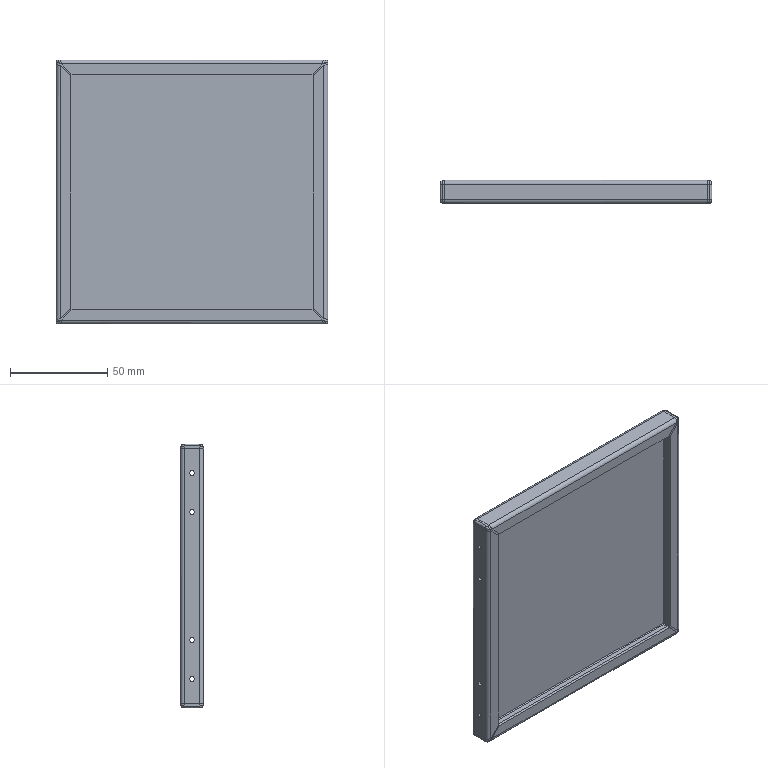Part | SolidWorks | features SMWeldBead 4, EdgeFlange 2, FlatPattern 1, HoleWzd 1, LPattern 1, MirrorPattern 1, SMBaseFlange 1, SheetMetal 1 | 1 solid | 130 faces | box 140 x 12 x 136 mm | volume 40853 mm3 | plane 54 | spline 40 | cylinder 36 | commonest cylinder face diameters 2.5 x16 1 x8 4 x8 2 x4